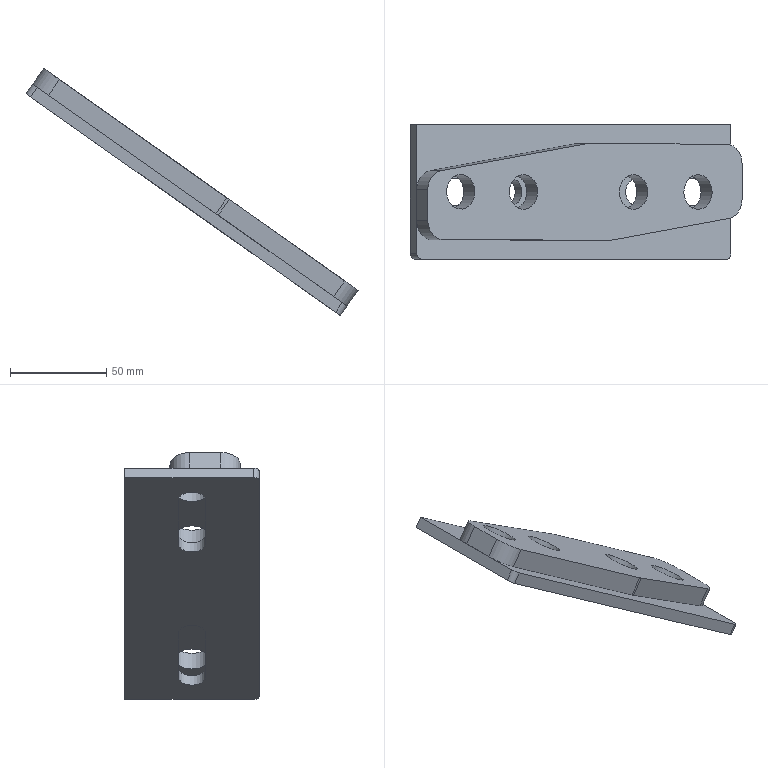Part | STEP file | tensioning conveyor mechanism lower bracket left 00 | 2 solids | 34 faces | box 172.614 x 70 x 128.419 mm | volume 151635 mm3 | plane 18 | cylinder 16 | commonest cylinder face diameters 20 x6 14 x4 18 x4 6 x2